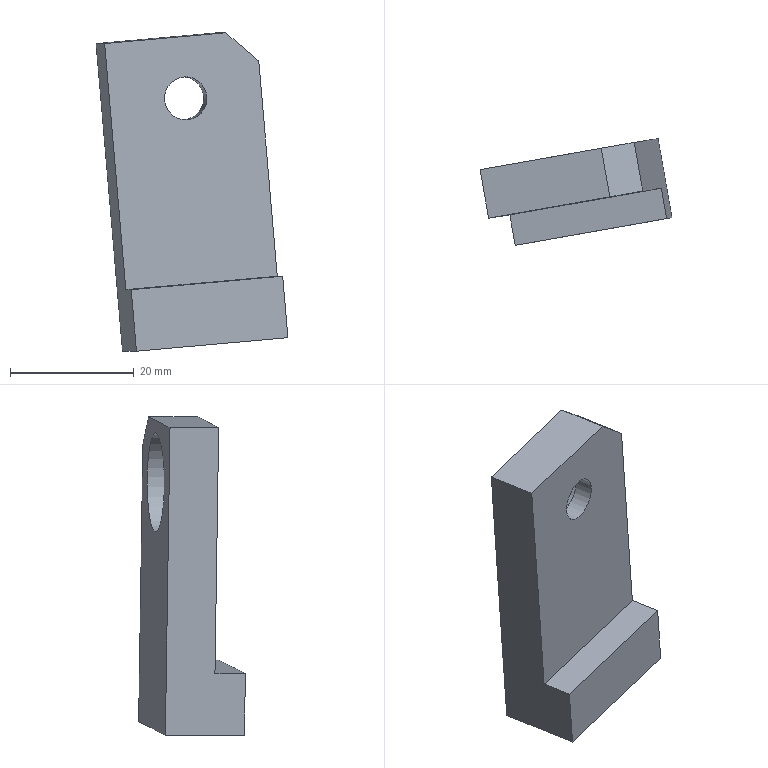Part | NX | features solid 2 | 1 solid | 12 faces | box 31.076 x 17.279 x 51.553 mm | volume 10031 mm3 | plane 10 | spline 2
STEP:
#1=CARTESIAN_POINT('',(1652.62,633.6,-6.91));
#2=VERTEX_POINT('',#1);
#3=CARTESIAN_POINT('',(1651.98,633.487,-8.698));
#4=CARTESIAN_POINT('',(1653.261,633.713,-5.123));
#5=CARTESIAN_POINT('',(1655.278,634.069,-4.168));
#6=CARTESIAN_POINT('',(1658.799,634.69,-5.469));
#7=CARTESIAN_POINT('',(1659.739,634.856,-7.517));
#8=CARTESIAN_POINT('',(1658.458,634.63,-11.092));
#9=CARTESIAN_POINT('',(1656.441,634.274,-12.047));
#10=CARTESIAN_POINT('',(1652.92,633.653,-10.746));
#11=CARTESIAN_POINT('',(1651.98,633.487,-8.698));
#12=CARTESIAN_POINT('',(1653.261,633.713,-5.123));
#13=B_SPLINE_CURVE_WITH_KNOTS('',3,(#3,#4,#5,#6,#7,#8,#9,#10,#11,#12),.UNSPECIFIED.,.T.,.F.,(2,2,2,2,2,2,2),(-0.25,0.,0.25,0.5,0.75,1.,1.25),.UNSPECIFIED.);
#14=EDGE_CURVE('',#2,#2,#13,.T.);
#15=ORIENTED_EDGE('',*,*,#14,.T.);
#16=EDGE_LOOP('',(#15));
#17=FACE_BOUND('',#16,.T.);
#18=CARTESIAN_POINT('',(1670.698,636.788,-36.904));
#19=VERTEX_POINT('',#18);
#20=CARTESIAN_POINT('',(1646.171,632.463,-39.083));
#21=VERTEX_POINT('',#20);
#22=CARTESIAN_POINT('',(1670.698,636.788,-36.904));
#23=CARTESIAN_POINT('',(1662.522,635.346,-37.63));
#24=CARTESIAN_POINT('',(1654.347,633.905,-38.357));
#25=CARTESIAN_POINT('',(1646.171,632.463,-39.083));
#26=B_SPLINE_CURVE_WITH_KNOTS('',3,(#22,#23,#24,#25),.UNSPECIFIED.,.F.,.F.,(4,4),(0.,1.),.PIECEWISE_BEZIER_KNOTS.);
#27=EDGE_CURVE('',#19,#21,#26,.T.);
#28=ORIENTED_EDGE('',*,*,#27,.F.);
#29=CARTESIAN_POINT('',(1667.693,636.258,-2.037));
#30=VERTEX_POINT('',#29);
#31=CARTESIAN_POINT('',(1668.981,636.485,-16.98));
#32=DIRECTION('',(-0.08583,-0.01513,0.9962));
#33=VECTOR('',#32,1000.);
#34=LINE('',#31,#33);
#35=EDGE_CURVE('',#19,#30,#34,.T.);
#36=ORIENTED_EDGE('',*,*,#35,.T.);
#37=CARTESIAN_POINT('',(1662.359,635.318,2.508));
#38=VERTEX_POINT('',#37);
#39=CARTESIAN_POINT('',(1667.693,636.258,-2.037));
#40=DIRECTION('',(-0.7544,-0.133,0.6428));
#41=VECTOR('',#40,1000.);
#42=LINE('',#39,#41);
#43=EDGE_CURVE('',#30,#38,#42,.T.);
#44=ORIENTED_EDGE('',*,*,#43,.T.);
#45=CARTESIAN_POINT('',(1642.738,631.858,0.765));
#46=VERTEX_POINT('',#45);
#47=CARTESIAN_POINT('',(1642.738,631.858,0.765));
#48=DIRECTION('',(0.9811,0.173,0.08716));
#49=VECTOR('',#48,1000.);
#50=LINE('',#47,#49);
#51=EDGE_CURVE('',#46,#38,#50,.T.);
#52=ORIENTED_EDGE('',*,*,#51,.F.);
#53=CARTESIAN_POINT('',(1647.029,632.614,-49.045));
#54=DIRECTION('',(-0.08583,-0.01513,0.9962));
#55=VECTOR('',#54,1000.);
#56=LINE('',#53,#55);
#57=EDGE_CURVE('',#21,#46,#56,.T.);
#58=ORIENTED_EDGE('',*,*,#57,.F.);
#59=EDGE_LOOP('',(#28,#36,#44,#52,#58));
#60=FACE_BOUND('',#59,.T.);
#61=CARTESIAN_POINT('',(1641.021,631.555,20.689));
#62=DIRECTION('',(-0.1736,0.9848,0.));
#63=DIRECTION('',(-0.8925,-0.1574,0.4226));
#64=AXIS2_PLACEMENT_3D('',#61,#62,#63);
#65=PLANE('',#64);
#66=ADVANCED_FACE('',(#17,#60),#65,.F.);
#67=CARTESIAN_POINT('',(1666.304,644.137,-2.037));
#68=VERTEX_POINT('',#67);
#69=CARTESIAN_POINT('',(1660.97,643.196,2.508));
#70=VERTEX_POINT('',#69);
#71=CARTESIAN_POINT('',(1666.304,644.137,-2.037));
#72=DIRECTION('',(-0.7544,-0.133,0.6428));
#73=VECTOR('',#72,1000.);
#74=LINE('',#71,#73);
#75=EDGE_CURVE('',#68,#70,#74,.T.);
#76=ORIENTED_EDGE('',*,*,#75,.T.);
#77=CARTESIAN_POINT('',(1662.359,635.318,2.508));
#78=DIRECTION('',(-0.1736,0.9848,0.));
#79=VECTOR('',#78,1000.);
#80=LINE('',#77,#79);
#81=EDGE_CURVE('',#38,#70,#80,.T.);
#82=ORIENTED_EDGE('',*,*,#81,.F.);
#83=ORIENTED_EDGE('',*,*,#43,.F.);
#84=CARTESIAN_POINT('',(1667.693,636.258,-2.037));
#85=DIRECTION('',(-0.1736,0.9848,0.));
#86=VECTOR('',#85,1000.);
#87=LINE('',#84,#86);
#88=EDGE_CURVE('',#30,#68,#87,.T.);
#89=ORIENTED_EDGE('',*,*,#88,.T.);
#90=EDGE_LOOP('',(#76,#82,#83,#89));
#91=FACE_BOUND('',#90,.T.);
#92=CARTESIAN_POINT('',(1667.693,636.258,-2.037));
#93=DIRECTION('',(-0.633,-0.1116,-0.766));
#94=DIRECTION('',(-0.7544,-0.133,0.6428));
#95=AXIS2_PLACEMENT_3D('',#92,#93,#94);
#96=PLANE('',#95);
#97=ADVANCED_FACE('',(#91),#96,.F.);
#98=CARTESIAN_POINT('',(1641.349,639.736,0.765));
#99=VERTEX_POINT('',#98);
#100=CARTESIAN_POINT('',(1641.349,639.736,0.765));
#101=DIRECTION('',(0.9811,0.173,0.08716));
#102=VECTOR('',#101,1000.);
#103=LINE('',#100,#102);
#104=EDGE_CURVE('',#99,#70,#103,.T.);
#105=ORIENTED_EDGE('',*,*,#104,.F.);
#106=CARTESIAN_POINT('',(1642.738,631.858,0.765));
#107=DIRECTION('',(-0.1736,0.9848,0.));
#108=VECTOR('',#107,1000.);
#109=LINE('',#106,#108);
#110=EDGE_CURVE('',#46,#99,#109,.T.);
#111=ORIENTED_EDGE('',*,*,#110,.F.);
#112=ORIENTED_EDGE('',*,*,#51,.T.);
#113=ORIENTED_EDGE('',*,*,#81,.T.);
#114=EDGE_LOOP('',(#105,#111,#112,#113));
#115=FACE_BOUND('',#114,.T.);
#116=CARTESIAN_POINT('',(1642.738,631.858,0.765));
#117=DIRECTION('',(-0.08583,-0.01513,0.9962));
#118=DIRECTION('',(0.9811,0.173,0.08716));
#119=AXIS2_PLACEMENT_3D('',#116,#117,#118);
#120=PLANE('',#119);
#121=ADVANCED_FACE('',(#115),#120,.T.);
#122=CARTESIAN_POINT('',(1645.64,640.493,-49.045));
#123=VERTEX_POINT('',#122);
#124=CARTESIAN_POINT('',(1645.64,640.493,-49.045));
#125=DIRECTION('',(-0.08583,-0.01513,0.9962));
#126=VECTOR('',#125,1000.);
#127=LINE('',#124,#126);
#128=EDGE_CURVE('',#123,#99,#127,.T.);
#129=ORIENTED_EDGE('',*,*,#128,.F.);
#130=CARTESIAN_POINT('',(1647.898,627.69,-49.045));
#131=VERTEX_POINT('',#130);
#132=CARTESIAN_POINT('',(1647.029,632.614,-49.045));
#133=DIRECTION('',(-0.1736,0.9848,0.));
#134=VECTOR('',#133,1000.);
#135=LINE('',#132,#134);
#136=EDGE_CURVE('',#131,#123,#135,.T.);
#137=ORIENTED_EDGE('',*,*,#136,.F.);
#138=CARTESIAN_POINT('',(1647.039,627.539,-39.083));
#139=VERTEX_POINT('',#138);
#140=CARTESIAN_POINT('',(1647.039,627.539,-39.083));
#141=DIRECTION('',(0.08583,0.01513,-0.9962));
#142=VECTOR('',#141,1000.);
#143=LINE('',#140,#142);
#144=EDGE_CURVE('',#139,#131,#143,.T.);
#145=ORIENTED_EDGE('',*,*,#144,.F.);
#146=CARTESIAN_POINT('',(1647.039,627.539,-39.083));
#147=DIRECTION('',(-0.1736,0.9848,0.));
#148=VECTOR('',#147,1000.);
#149=LINE('',#146,#148);
#150=EDGE_CURVE('',#139,#21,#149,.T.);
#151=ORIENTED_EDGE('',*,*,#150,.T.);
#152=ORIENTED_EDGE('',*,*,#57,.T.);
#153=ORIENTED_EDGE('',*,*,#110,.T.);
#154=EDGE_LOOP('',(#129,#137,#145,#151,#152,#153));
#155=FACE_BOUND('',#154,.T.);
#156=CARTESIAN_POINT('',(1647.029,632.614,-49.045));
#157=DIRECTION('',(-0.9811,-0.173,-0.08716));
#158=DIRECTION('',(-0.08583,-0.01513,0.9962));
#159=AXIS2_PLACEMENT_3D('',#156,#157,#158);
#160=PLANE('',#159);
#161=ADVANCED_FACE('',(#155),#160,.T.);
#162=CARTESIAN_POINT('',(1670.167,644.818,-46.866));
#163=VERTEX_POINT('',#162);
#164=CARTESIAN_POINT('',(1670.167,644.818,-46.866));
#165=DIRECTION('',(-0.9811,-0.173,-0.08716));
#166=VECTOR('',#165,1000.);
#167=LINE('',#164,#166);
#168=EDGE_CURVE('',#163,#123,#167,.T.);
#169=ORIENTED_EDGE('',*,*,#168,.F.);
#170=CARTESIAN_POINT('',(1672.424,632.015,-46.866));
#171=VERTEX_POINT('',#170);
#172=CARTESIAN_POINT('',(1671.556,636.939,-46.866));
#173=DIRECTION('',(-0.1736,0.9848,0.));
#174=VECTOR('',#173,1000.);
#175=LINE('',#172,#174);
#176=EDGE_CURVE('',#171,#163,#175,.T.);
#177=ORIENTED_EDGE('',*,*,#176,.F.);
#178=CARTESIAN_POINT('',(1672.424,632.015,-46.866));
#179=DIRECTION('',(-0.9811,-0.173,-0.08716));
#180=VECTOR('',#179,1000.);
#181=LINE('',#178,#180);
#182=EDGE_CURVE('',#171,#131,#181,.T.);
#183=ORIENTED_EDGE('',*,*,#182,.T.);
#184=ORIENTED_EDGE('',*,*,#136,.T.);
#185=EDGE_LOOP('',(#169,#177,#183,#184));
#186=FACE_BOUND('',#185,.T.);
#187=CARTESIAN_POINT('',(1671.556,636.939,-46.866));
#188=DIRECTION('',(0.08583,0.01513,-0.9962));
#189=DIRECTION('',(-0.9811,-0.173,-0.08716));
#190=AXIS2_PLACEMENT_3D('',#187,#188,#189);
#191=PLANE('',#190);
#192=ADVANCED_FACE('',(#186),#191,.T.);
#193=CARTESIAN_POINT('',(1667.592,644.364,-16.98));
#194=DIRECTION('',(-0.08583,-0.01513,0.9962));
#195=VECTOR('',#194,1000.);
#196=LINE('',#193,#195);
#197=EDGE_CURVE('',#163,#68,#196,.T.);
#198=ORIENTED_EDGE('',*,*,#197,.T.);
#199=ORIENTED_EDGE('',*,*,#88,.F.);
#200=ORIENTED_EDGE('',*,*,#35,.F.);
#201=CARTESIAN_POINT('',(1671.566,631.864,-36.904));
#202=VERTEX_POINT('',#201);
#203=CARTESIAN_POINT('',(1671.566,631.864,-36.904));
#204=DIRECTION('',(-0.1736,0.9848,0.));
#205=VECTOR('',#204,1000.);
#206=LINE('',#203,#205);
#207=EDGE_CURVE('',#202,#19,#206,.T.);
#208=ORIENTED_EDGE('',*,*,#207,.F.);
#209=CARTESIAN_POINT('',(1671.566,631.864,-36.904));
#210=DIRECTION('',(0.08583,0.01513,-0.9962));
#211=VECTOR('',#210,1000.);
#212=LINE('',#209,#211);
#213=EDGE_CURVE('',#202,#171,#212,.T.);
#214=ORIENTED_EDGE('',*,*,#213,.T.);
#215=ORIENTED_EDGE('',*,*,#176,.T.);
#216=EDGE_LOOP('',(#198,#199,#200,#208,#214,#215));
#217=FACE_BOUND('',#216,.T.);
#218=CARTESIAN_POINT('',(1668.981,636.485,-16.98));
#219=DIRECTION('',(-0.9811,-0.173,-0.08716));
#220=DIRECTION('',(-0.08583,-0.01513,0.9962));
#221=AXIS2_PLACEMENT_3D('',#218,#219,#220);
#222=PLANE('',#221);
#223=ADVANCED_FACE('',(#217),#222,.F.);
#224=CARTESIAN_POINT('',(1647.067,640.745,-5.371));
#225=VERTEX_POINT('',#224);
#226=CARTESIAN_POINT('',(1646.357,640.619,-7.351));
#227=CARTESIAN_POINT('',(1647.777,640.87,-3.391));
#228=CARTESIAN_POINT('',(1649.26,641.131,-1.748));
#229=CARTESIAN_POINT('',(1653.021,641.794,0.03336));
#230=CARTESIAN_POINT('',(1655.215,642.181,0.1306));
#231=CARTESIAN_POINT('',(1659.115,642.869,-1.311));
#232=CARTESIAN_POINT('',(1660.734,643.154,-2.817));
#233=CARTESIAN_POINT('',(1662.487,643.464,-6.636));
#234=CARTESIAN_POINT('',(1662.583,643.48,-8.864));
#235=CARTESIAN_POINT('',(1661.164,643.23,-12.824));
#236=CARTESIAN_POINT('',(1659.68,642.969,-14.468));
#237=CARTESIAN_POINT('',(1655.919,642.305,-16.248));
#238=CARTESIAN_POINT('',(1653.725,641.919,-16.346));
#239=CARTESIAN_POINT('',(1649.826,641.231,-14.904));
#240=CARTESIAN_POINT('',(1648.207,640.946,-13.398));
#241=CARTESIAN_POINT('',(1646.453,640.636,-9.579));
#242=CARTESIAN_POINT('',(1646.357,640.619,-7.351));
#243=CARTESIAN_POINT('',(1647.777,640.87,-3.391));
#244=B_SPLINE_CURVE_WITH_KNOTS('',3,(#226,#227,#228,#229,#230,#231,#232,#233,#234,#235,#236,#237,#238,#239,#240,#241,#242,#243),.UNSPECIFIED.,.T.,.F.,(2,2,2,2,2,2,2,2,2,2,2),(-0.125,0.,0.125,0.25,0.375,0.5,0.625,0.75,0.875,1.,1.125),.UNSPECIFIED.);
#245=EDGE_CURVE('',#225,#225,#244,.T.);
#246=ORIENTED_EDGE('',*,*,#245,.F.);
#247=EDGE_LOOP('',(#246));
#248=FACE_BOUND('',#247,.T.);
#249=ORIENTED_EDGE('',*,*,#75,.F.);
#250=ORIENTED_EDGE('',*,*,#197,.F.);
#251=ORIENTED_EDGE('',*,*,#168,.T.);
#252=ORIENTED_EDGE('',*,*,#128,.T.);
#253=ORIENTED_EDGE('',*,*,#104,.T.);
#254=EDGE_LOOP('',(#249,#250,#251,#252,#253));
#255=FACE_BOUND('',#254,.T.);
#256=CARTESIAN_POINT('',(1639.632,639.434,20.689));
#257=DIRECTION('',(-0.1736,0.9848,0.));
#258=DIRECTION('',(-0.8925,-0.1574,0.4226));
#259=AXIS2_PLACEMENT_3D('',#256,#257,#258);
#260=PLANE('',#259);
#261=ADVANCED_FACE('',(#248,#255),#260,.T.);
#262=CARTESIAN_POINT('',(1647.935,635.82,-5.371));
#263=VERTEX_POINT('',#262);
#264=CARTESIAN_POINT('',(1647.225,635.695,-7.351));
#265=CARTESIAN_POINT('',(1648.645,635.946,-3.391));
#266=CARTESIAN_POINT('',(1650.128,636.207,-1.748));
#267=CARTESIAN_POINT('',(1653.889,636.87,0.03336));
#268=CARTESIAN_POINT('',(1656.083,637.257,0.1306));
#269=CARTESIAN_POINT('',(1659.983,637.945,-1.311));
#270=CARTESIAN_POINT('',(1661.602,638.23,-2.817));
#271=CARTESIAN_POINT('',(1663.356,638.54,-6.636));
#272=CARTESIAN_POINT('',(1663.451,638.556,-8.864));
#273=CARTESIAN_POINT('',(1662.032,638.306,-12.824));
#274=CARTESIAN_POINT('',(1660.549,638.045,-14.468));
#275=CARTESIAN_POINT('',(1656.787,637.381,-16.248));
#276=CARTESIAN_POINT('',(1654.594,636.995,-16.346));
#277=CARTESIAN_POINT('',(1650.694,636.307,-14.904));
#278=CARTESIAN_POINT('',(1649.075,636.021,-13.398));
#279=CARTESIAN_POINT('',(1647.321,635.712,-9.579));
#280=CARTESIAN_POINT('',(1647.225,635.695,-7.351));
#281=CARTESIAN_POINT('',(1648.645,635.946,-3.391));
#282=B_SPLINE_CURVE_WITH_KNOTS('',3,(#264,#265,#266,#267,#268,#269,#270,#271,#272,#273,#274,#275,#276,#277,#278,#279,#280,#281),.UNSPECIFIED.,.T.,.F.,(2,2,2,2,2,2,2,2,2,2,2),(-0.125,0.,0.125,0.25,0.375,0.5,0.625,0.75,0.875,1.,1.125),.UNSPECIFIED.);
#283=EDGE_CURVE('',#263,#263,#282,.T.);
#284=ORIENTED_EDGE('',*,*,#283,.F.);
#285=EDGE_LOOP('',(#284));
#286=FACE_BOUND('',#285,.T.);
#287=ORIENTED_EDGE('',*,*,#245,.T.);
#288=EDGE_LOOP('',(#287));
#289=FACE_BOUND('',#288,.T.);
#290=CARTESIAN_POINT('',(1647.426,635.731,-11.854));
#291=CARTESIAN_POINT('',(1646.557,640.655,-11.854));
#292=CARTESIAN_POINT('',(1647.134,635.679,-5.075));
#293=CARTESIAN_POINT('',(1646.266,640.603,-5.075));
#294=CARTESIAN_POINT('',(1651.649,636.475,-0.07261));
#295=CARTESIAN_POINT('',(1650.78,641.399,-0.07261));
#296=CARTESIAN_POINT('',(1658.325,637.652,0.2234));
#297=CARTESIAN_POINT('',(1657.456,642.576,0.2234));
#298=CARTESIAN_POINT('',(1663.251,638.521,-4.361));
#299=CARTESIAN_POINT('',(1662.383,643.445,-4.361));
#300=CARTESIAN_POINT('',(1663.543,638.573,-11.14));
#301=CARTESIAN_POINT('',(1662.675,643.497,-11.14));
#302=CARTESIAN_POINT('',(1659.028,637.776,-16.142));
#303=CARTESIAN_POINT('',(1658.16,642.701,-16.142));
#304=CARTESIAN_POINT('',(1652.352,636.599,-16.438));
#305=CARTESIAN_POINT('',(1651.484,641.523,-16.438));
#306=CARTESIAN_POINT('',(1647.426,635.731,-11.854));
#307=CARTESIAN_POINT('',(1646.557,640.655,-11.854));
#308=CARTESIAN_POINT('',(1647.134,635.679,-5.075));
#309=CARTESIAN_POINT('',(1646.266,640.603,-5.075));
#310=CARTESIAN_POINT('',(1651.649,636.475,-0.07261));
#311=CARTESIAN_POINT('',(1650.78,641.399,-0.07261));
#312=B_SPLINE_SURFACE_WITH_KNOTS('',3,1,((#290,#291),(#292,#293),(#294,#295),(#296,#297),(#298,#299),(#300,#301),(#302,#303),(#304,#305),(#306,#307),(#308,#309),(#310,#311)),.SURF_OF_LINEAR_EXTRUSION.,.T.,.F.,.F.,(1,1,1,1,1,1,1,1,1,1,1,1,1,1,1),(2,2),(-0.375,-0.25,-0.125,0.,0.125,0.25,0.375,0.5,0.625,0.75,0.875,1.,1.125,1.25,1.375),(0.,1.),.UNSPECIFIED.);
#313=ADVANCED_FACE('',(#286,#289),#312,.F.);
#314=CARTESIAN_POINT('',(1652.099,636.555,-6.91));
#315=VERTEX_POINT('',#314);
#316=CARTESIAN_POINT('',(1651.459,636.442,-8.698));
#317=CARTESIAN_POINT('',(1652.74,636.668,-5.123));
#318=CARTESIAN_POINT('',(1654.757,637.023,-4.168));
#319=CARTESIAN_POINT('',(1658.278,637.644,-5.469));
#320=CARTESIAN_POINT('',(1659.218,637.81,-7.517));
#321=CARTESIAN_POINT('',(1657.937,637.584,-11.092));
#322=CARTESIAN_POINT('',(1655.92,637.228,-12.047));
#323=CARTESIAN_POINT('',(1652.399,636.608,-10.746));
#324=CARTESIAN_POINT('',(1651.459,636.442,-8.698));
#325=CARTESIAN_POINT('',(1652.74,636.668,-5.123));
#326=B_SPLINE_CURVE_WITH_KNOTS('',3,(#316,#317,#318,#319,#320,#321,#322,#323,#324,#325),.UNSPECIFIED.,.T.,.F.,(2,2,2,2,2,2,2),(-0.25,0.,0.25,0.5,0.75,1.,1.25),.UNSPECIFIED.);
#327=EDGE_CURVE('',#315,#315,#326,.F.);
#328=ORIENTED_EDGE('',*,*,#327,.T.);
#329=EDGE_LOOP('',(#328));
#330=FACE_BOUND('',#329,.T.);
#331=ORIENTED_EDGE('',*,*,#283,.T.);
#332=EDGE_LOOP('',(#331));
#333=FACE_BOUND('',#332,.T.);
#334=CARTESIAN_POINT('',(1662.742,638.431,-10.844));
#335=DIRECTION('',(0.1736,-0.9848,0.));
#336=DIRECTION('',(0.8925,0.1574,-0.4226));
#337=AXIS2_PLACEMENT_3D('',#334,#335,#336);
#338=PLANE('',#337);
#339=ADVANCED_FACE('',(#330,#333),#338,.F.);
#340=ORIENTED_EDGE('',*,*,#14,.F.);
#341=EDGE_LOOP('',(#340));
#342=FACE_BOUND('',#341,.T.);
#343=ORIENTED_EDGE('',*,*,#327,.F.);
#344=EDGE_LOOP('',(#343));
#345=FACE_BOUND('',#344,.T.);
#346=CARTESIAN_POINT('',(1652.423,633.565,-9.735));
#347=CARTESIAN_POINT('',(1651.902,636.52,-9.735));
#348=CARTESIAN_POINT('',(1652.261,633.537,-6.778));
#349=CARTESIAN_POINT('',(1651.74,636.491,-6.778));
#350=CARTESIAN_POINT('',(1654.257,633.889,-4.618));
#351=CARTESIAN_POINT('',(1653.736,636.843,-4.618));
#352=CARTESIAN_POINT('',(1657.169,634.402,-4.453));
#353=CARTESIAN_POINT('',(1656.648,637.357,-4.453));
#354=CARTESIAN_POINT('',(1659.296,634.777,-6.48));
#355=CARTESIAN_POINT('',(1658.775,637.732,-6.48));
#356=CARTESIAN_POINT('',(1659.458,634.806,-9.438));
#357=CARTESIAN_POINT('',(1658.937,637.76,-9.438));
#358=CARTESIAN_POINT('',(1657.462,634.454,-11.597));
#359=CARTESIAN_POINT('',(1656.941,637.408,-11.597));
#360=CARTESIAN_POINT('',(1654.55,633.941,-11.762));
#361=CARTESIAN_POINT('',(1654.029,636.895,-11.762));
#362=CARTESIAN_POINT('',(1652.423,633.565,-9.735));
#363=CARTESIAN_POINT('',(1651.902,636.52,-9.735));
#364=CARTESIAN_POINT('',(1652.261,633.537,-6.778));
#365=CARTESIAN_POINT('',(1651.74,636.491,-6.778));
#366=CARTESIAN_POINT('',(1654.257,633.889,-4.618));
#367=CARTESIAN_POINT('',(1653.736,636.843,-4.618));
#368=B_SPLINE_SURFACE_WITH_KNOTS('',3,1,((#346,#347),(#348,#349),(#350,#351),(#352,#353),(#354,#355),(#356,#357),(#358,#359),(#360,#361),(#362,#363),(#364,#365),(#366,#367)),.SURF_OF_LINEAR_EXTRUSION.,.T.,.F.,.F.,(1,1,1,1,1,1,1,1,1,1,1,1,1,1,1),(2,2),(-0.375,-0.25,-0.125,0.,0.125,0.25,0.375,0.5,0.625,0.75,0.875,1.,1.125,1.25,1.375),(0.,1.),.UNSPECIFIED.);
#369=ADVANCED_FACE('',(#342,#345),#368,.F.);
#370=ORIENTED_EDGE('',*,*,#27,.T.);
#371=ORIENTED_EDGE('',*,*,#150,.F.);
#372=CARTESIAN_POINT('',(1671.566,631.864,-36.904));
#373=CARTESIAN_POINT('',(1663.39,630.422,-37.63));
#374=CARTESIAN_POINT('',(1655.215,628.981,-38.357));
#375=CARTESIAN_POINT('',(1647.039,627.539,-39.083));
#376=B_SPLINE_CURVE_WITH_KNOTS('',3,(#372,#373,#374,#375),.UNSPECIFIED.,.F.,.F.,(4,4),(0.,1.),.PIECEWISE_BEZIER_KNOTS.);
#377=EDGE_CURVE('',#202,#139,#376,.T.);
#378=ORIENTED_EDGE('',*,*,#377,.F.);
#379=ORIENTED_EDGE('',*,*,#207,.T.);
#380=EDGE_LOOP('',(#370,#371,#378,#379));
#381=FACE_BOUND('',#380,.T.);
#382=CARTESIAN_POINT('',(1671.566,631.864,-36.904));
#383=DIRECTION('',(0.08583,0.01513,-0.9962));
#384=DIRECTION('',(-0.9811,-0.173,-0.08716));
#385=AXIS2_PLACEMENT_3D('',#382,#383,#384);
#386=PLANE('',#385);
#387=ADVANCED_FACE('',(#381),#386,.F.);
#388=ORIENTED_EDGE('',*,*,#182,.F.);
#389=ORIENTED_EDGE('',*,*,#213,.F.);
#390=ORIENTED_EDGE('',*,*,#377,.T.);
#391=ORIENTED_EDGE('',*,*,#144,.T.);
#392=EDGE_LOOP('',(#388,#389,#390,#391));
#393=FACE_BOUND('',#392,.T.);
#394=CARTESIAN_POINT('',(1672.424,632.015,-46.866));
#395=DIRECTION('',(-0.1736,0.9848,0.));
#396=DIRECTION('',(-0.8925,-0.1574,0.4226));
#397=AXIS2_PLACEMENT_3D('',#394,#395,#396);
#398=PLANE('',#397);
#399=ADVANCED_FACE('',(#393),#398,.F.);
#400=CLOSED_SHELL('',(#66,#97,#121,#161,#192,#223,#261,#313,#339,#369,#387,#399));
#401=MANIFOLD_SOLID_BREP('',#400);
#402=(LENGTH_UNIT()NAMED_UNIT(*)SI_UNIT(.MILLI.,.METRE.));
#403=UNCERTAINTY_MEASURE_WITH_UNIT(LENGTH_MEASURE(0.0508),#402,'','');
#404=(NAMED_UNIT(*)PLANE_ANGLE_UNIT()SI_UNIT($,.RADIAN.));
#405=(NAMED_UNIT(*)SI_UNIT($,.STERADIAN.)SOLID_ANGLE_UNIT());
#406=(GEOMETRIC_REPRESENTATION_CONTEXT(3)GLOBAL_UNCERTAINTY_ASSIGNED_CONTEXT((#403))GLOBAL_UNIT_ASSIGNED_CONTEXT((#402,#404,#405))REPRESENTATION_CONTEXT('',''));
#407=ADVANCED_BREP_SHAPE_REPRESENTATION('',(#401),#406);